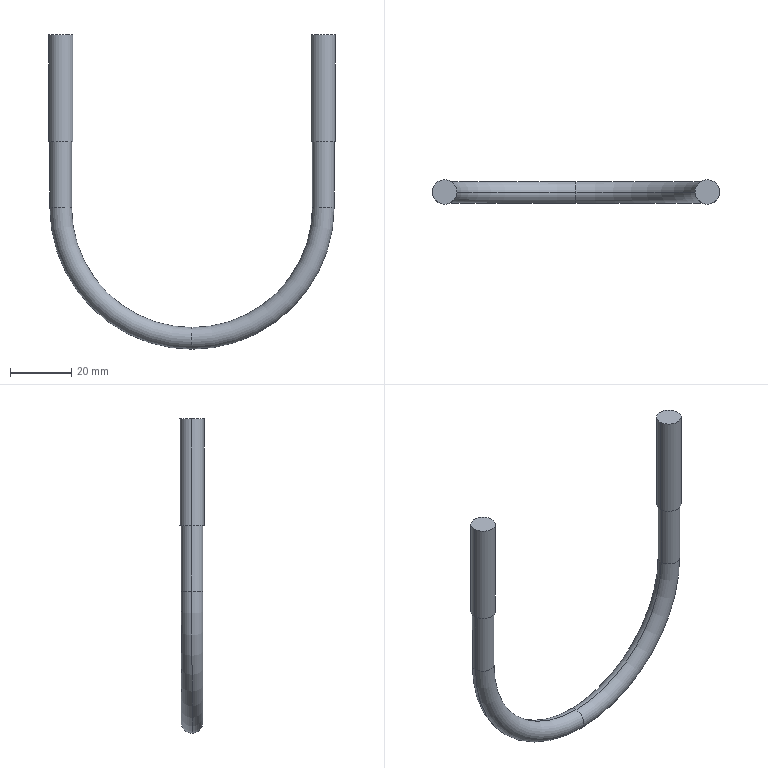Part | SolidWorks | features ICE 1, Sweep 1 | 1 solid | 16 faces | box 94 x 8 x 103 mm | volume 10565 mm3 | cylinder 8 | torus 4 | plane 4 | commonest cylinder face diameters 7.1 x4 8 x4
STEP:
#1=CARTESIAN_POINT('',(43.,0.,-103.));
#2=VERTEX_POINT('',#1);
#3=CARTESIAN_POINT('',(43.,0.,-95.9));
#4=VERTEX_POINT('',#3);
#5=CARTESIAN_POINT('',(43.,0.,-99.45));
#6=DIRECTION('',(-1.,0.,0.));
#7=DIRECTION('',(0.,0.,1.));
#8=AXIS2_PLACEMENT_3D('',#5,#6,#7);
#9=CIRCLE('',#8,3.55);
#10=EDGE_CURVE('',#2,#4,#9,.T.);
#11=ORIENTED_EDGE('',*,*,#10,.F.);
#12=CARTESIAN_POINT('',(89.55,0.,-56.45));
#13=VERTEX_POINT('',#12);
#14=CARTESIAN_POINT('',(43.,0.,-56.45));
#15=DIRECTION('',(0.,-1.,0.));
#16=DIRECTION('',(0.,0.,-1.));
#17=AXIS2_PLACEMENT_3D('',#14,#15,#16);
#18=CIRCLE('',#17,46.55);
#19=EDGE_CURVE('',#2,#13,#18,.T.);
#20=ORIENTED_EDGE('',*,*,#19,.T.);
#21=CARTESIAN_POINT('',(82.45,0.,-56.45));
#22=VERTEX_POINT('',#21);
#23=CARTESIAN_POINT('',(86.,0.,-56.45));
#24=DIRECTION('',(0.,0.,-1.));
#25=DIRECTION('',(-1.,0.,0.));
#26=AXIS2_PLACEMENT_3D('',#23,#24,#25);
#27=CIRCLE('',#26,3.55);
#28=EDGE_CURVE('',#13,#22,#27,.T.);
#29=ORIENTED_EDGE('',*,*,#28,.T.);
#30=CARTESIAN_POINT('',(43.,0.,-56.45));
#31=DIRECTION('',(0.,-1.,0.));
#32=DIRECTION('',(0.,0.,-1.));
#33=AXIS2_PLACEMENT_3D('',#30,#31,#32);
#34=CIRCLE('',#33,39.45);
#35=EDGE_CURVE('',#4,#22,#34,.T.);
#36=ORIENTED_EDGE('',*,*,#35,.F.);
#37=EDGE_LOOP('',(#11,#20,#29,#36));
#38=FACE_OUTER_BOUND('',#37,.T.);
#39=CARTESIAN_POINT('',(43.,0.,-56.45));
#40=DIRECTION('',(0.,-1.,0.));
#41=DIRECTION('',(0.,0.,-1.));
#42=AXIS2_PLACEMENT_3D('',#39,#40,#41);
#43=TOROIDAL_SURFACE('',#42,43.,3.55);
#44=ADVANCED_FACE('',(#38),#43,.T.);
#45=CARTESIAN_POINT('',(-3.55,0.,-56.45));
#46=VERTEX_POINT('',#45);
#47=CARTESIAN_POINT('',(3.55,0.,-56.45));
#48=VERTEX_POINT('',#47);
#49=CARTESIAN_POINT('',(0.,0.,-56.45));
#50=DIRECTION('',(0.,0.,1.));
#51=DIRECTION('',(1.,0.,0.));
#52=AXIS2_PLACEMENT_3D('',#49,#50,#51);
#53=CIRCLE('',#52,3.55);
#54=EDGE_CURVE('',#46,#48,#53,.T.);
#55=ORIENTED_EDGE('',*,*,#54,.F.);
#56=CARTESIAN_POINT('',(43.,0.,-56.45));
#57=DIRECTION('',(0.,-1.,0.));
#58=DIRECTION('',(0.,0.,-1.));
#59=AXIS2_PLACEMENT_3D('',#56,#57,#58);
#60=CIRCLE('',#59,46.55);
#61=EDGE_CURVE('',#46,#2,#60,.T.);
#62=ORIENTED_EDGE('',*,*,#61,.T.);
#63=ORIENTED_EDGE('',*,*,#10,.T.);
#64=CARTESIAN_POINT('',(43.,0.,-56.45));
#65=DIRECTION('',(0.,-1.,0.));
#66=DIRECTION('',(0.,0.,-1.));
#67=AXIS2_PLACEMENT_3D('',#64,#65,#66);
#68=CIRCLE('',#67,39.45);
#69=EDGE_CURVE('',#48,#4,#68,.T.);
#70=ORIENTED_EDGE('',*,*,#69,.F.);
#71=EDGE_LOOP('',(#55,#62,#63,#70));
#72=FACE_OUTER_BOUND('',#71,.T.);
#73=CARTESIAN_POINT('',(43.,0.,-56.45));
#74=DIRECTION('',(0.,-1.,0.));
#75=DIRECTION('',(0.,0.,-1.));
#76=AXIS2_PLACEMENT_3D('',#73,#74,#75);
#77=TOROIDAL_SURFACE('',#76,43.,3.55);
#78=ADVANCED_FACE('',(#72),#77,.T.);
#79=CARTESIAN_POINT('',(90.,0.,-35.));
#80=VERTEX_POINT('',#79);
#81=CARTESIAN_POINT('',(82.,0.,-35.));
#82=VERTEX_POINT('',#81);
#83=CARTESIAN_POINT('',(86.,0.,-35.));
#84=DIRECTION('',(0.,0.,1.));
#85=DIRECTION('',(1.,0.,0.));
#86=AXIS2_PLACEMENT_3D('',#83,#84,#85);
#87=CIRCLE('',#86,4.);
#88=EDGE_CURVE('',#80,#82,#87,.T.);
#89=ORIENTED_EDGE('',*,*,#88,.T.);
#90=CARTESIAN_POINT('',(82.,0.,0.));
#91=VERTEX_POINT('',#90);
#92=CARTESIAN_POINT('',(82.,0.,-35.));
#93=DIRECTION('',(0.,0.,1.));
#94=VECTOR('',#93,1000.);
#95=LINE('',#92,#94);
#96=EDGE_CURVE('',#82,#91,#95,.T.);
#97=ORIENTED_EDGE('',*,*,#96,.T.);
#98=CARTESIAN_POINT('',(90.,0.,0.));
#99=VERTEX_POINT('',#98);
#100=CARTESIAN_POINT('',(86.,0.,0.));
#101=DIRECTION('',(0.,0.,1.));
#102=DIRECTION('',(1.,0.,0.));
#103=AXIS2_PLACEMENT_3D('',#100,#101,#102);
#104=CIRCLE('',#103,4.);
#105=EDGE_CURVE('',#99,#91,#104,.T.);
#106=ORIENTED_EDGE('',*,*,#105,.F.);
#107=CARTESIAN_POINT('',(90.,0.,-35.));
#108=DIRECTION('',(0.,0.,1.));
#109=VECTOR('',#108,1000.);
#110=LINE('',#107,#109);
#111=EDGE_CURVE('',#80,#99,#110,.T.);
#112=ORIENTED_EDGE('',*,*,#111,.F.);
#113=EDGE_LOOP('',(#89,#97,#106,#112));
#114=FACE_OUTER_BOUND('',#113,.T.);
#115=CARTESIAN_POINT('',(86.,0.,-35.));
#116=DIRECTION('',(0.,0.,1.));
#117=DIRECTION('',(1.,0.,0.));
#118=AXIS2_PLACEMENT_3D('',#115,#116,#117);
#119=CYLINDRICAL_SURFACE('',#118,4.);
#120=ADVANCED_FACE('',(#114),#119,.T.);
#121=CARTESIAN_POINT('',(4.,0.,-35.));
#122=VERTEX_POINT('',#121);
#123=CARTESIAN_POINT('',(-4.,0.,-35.));
#124=VERTEX_POINT('',#123);
#125=CARTESIAN_POINT('',(0.,0.,-35.));
#126=DIRECTION('',(0.,0.,1.));
#127=DIRECTION('',(1.,0.,0.));
#128=AXIS2_PLACEMENT_3D('',#125,#126,#127);
#129=CIRCLE('',#128,4.);
#130=EDGE_CURVE('',#122,#124,#129,.T.);
#131=ORIENTED_EDGE('',*,*,#130,.T.);
#132=CARTESIAN_POINT('',(-4.,0.,0.));
#133=VERTEX_POINT('',#132);
#134=CARTESIAN_POINT('',(-4.,0.,-35.));
#135=DIRECTION('',(0.,0.,1.));
#136=VECTOR('',#135,1000.);
#137=LINE('',#134,#136);
#138=EDGE_CURVE('',#124,#133,#137,.T.);
#139=ORIENTED_EDGE('',*,*,#138,.T.);
#140=CARTESIAN_POINT('',(4.,0.,0.));
#141=VERTEX_POINT('',#140);
#142=CARTESIAN_POINT('',(0.,0.,0.));
#143=DIRECTION('',(0.,0.,1.));
#144=DIRECTION('',(1.,0.,0.));
#145=AXIS2_PLACEMENT_3D('',#142,#143,#144);
#146=CIRCLE('',#145,4.);
#147=EDGE_CURVE('',#141,#133,#146,.T.);
#148=ORIENTED_EDGE('',*,*,#147,.F.);
#149=CARTESIAN_POINT('',(4.,0.,-35.));
#150=DIRECTION('',(0.,0.,1.));
#151=VECTOR('',#150,1000.);
#152=LINE('',#149,#151);
#153=EDGE_CURVE('',#122,#141,#152,.T.);
#154=ORIENTED_EDGE('',*,*,#153,.F.);
#155=EDGE_LOOP('',(#131,#139,#148,#154));
#156=FACE_OUTER_BOUND('',#155,.T.);
#157=CARTESIAN_POINT('',(0.,0.,-35.));
#158=DIRECTION('',(0.,0.,1.));
#159=DIRECTION('',(1.,0.,0.));
#160=AXIS2_PLACEMENT_3D('',#157,#158,#159);
#161=CYLINDRICAL_SURFACE('',#160,4.);
#162=ADVANCED_FACE('',(#156),#161,.T.);
#163=ORIENTED_EDGE('',*,*,#61,.F.);
#164=CARTESIAN_POINT('',(0.,0.,-56.45));
#165=DIRECTION('',(0.,0.,1.));
#166=DIRECTION('',(1.,0.,0.));
#167=AXIS2_PLACEMENT_3D('',#164,#165,#166);
#168=CIRCLE('',#167,3.55);
#169=EDGE_CURVE('',#48,#46,#168,.T.);
#170=ORIENTED_EDGE('',*,*,#169,.F.);
#171=ORIENTED_EDGE('',*,*,#69,.T.);
#172=CARTESIAN_POINT('',(43.,0.,-99.45));
#173=DIRECTION('',(-1.,0.,0.));
#174=DIRECTION('',(0.,0.,1.));
#175=AXIS2_PLACEMENT_3D('',#172,#173,#174);
#176=CIRCLE('',#175,3.55);
#177=EDGE_CURVE('',#4,#2,#176,.T.);
#178=ORIENTED_EDGE('',*,*,#177,.T.);
#179=EDGE_LOOP('',(#163,#170,#171,#178));
#180=FACE_OUTER_BOUND('',#179,.T.);
#181=CARTESIAN_POINT('',(43.,0.,-56.45));
#182=DIRECTION('',(0.,-1.,0.));
#183=DIRECTION('',(0.,0.,-1.));
#184=AXIS2_PLACEMENT_3D('',#181,#182,#183);
#185=TOROIDAL_SURFACE('',#184,43.,3.55);
#186=ADVANCED_FACE('',(#180),#185,.T.);
#187=CARTESIAN_POINT('',(3.55,0.,-35.));
#188=VERTEX_POINT('',#187);
#189=CARTESIAN_POINT('',(-3.55,0.,-35.));
#190=VERTEX_POINT('',#189);
#191=CARTESIAN_POINT('',(0.,0.,-35.));
#192=DIRECTION('',(0.,0.,1.));
#193=DIRECTION('',(1.,0.,0.));
#194=AXIS2_PLACEMENT_3D('',#191,#192,#193);
#195=CIRCLE('',#194,3.55);
#196=EDGE_CURVE('',#188,#190,#195,.T.);
#197=ORIENTED_EDGE('',*,*,#196,.F.);
#198=CARTESIAN_POINT('',(3.55,0.,0.));
#199=DIRECTION('',(0.,0.,-1.));
#200=VECTOR('',#199,1000.);
#201=LINE('',#198,#200);
#202=EDGE_CURVE('',#188,#48,#201,.T.);
#203=ORIENTED_EDGE('',*,*,#202,.T.);
#204=ORIENTED_EDGE('',*,*,#169,.T.);
#205=CARTESIAN_POINT('',(-3.55,0.,0.));
#206=DIRECTION('',(0.,0.,-1.));
#207=VECTOR('',#206,1000.);
#208=LINE('',#205,#207);
#209=EDGE_CURVE('',#190,#46,#208,.T.);
#210=ORIENTED_EDGE('',*,*,#209,.F.);
#211=EDGE_LOOP('',(#197,#203,#204,#210));
#212=FACE_OUTER_BOUND('',#211,.T.);
#213=CARTESIAN_POINT('',(0.,0.,0.));
#214=DIRECTION('',(0.,0.,-1.));
#215=DIRECTION('',(-1.,0.,0.));
#216=AXIS2_PLACEMENT_3D('',#213,#214,#215);
#217=CYLINDRICAL_SURFACE('',#216,3.55);
#218=ADVANCED_FACE('',(#212),#217,.T.);
#219=CARTESIAN_POINT('',(86.,0.,-56.45));
#220=DIRECTION('',(0.,0.,-1.));
#221=DIRECTION('',(-1.,0.,0.));
#222=AXIS2_PLACEMENT_3D('',#219,#220,#221);
#223=CIRCLE('',#222,3.55);
#224=EDGE_CURVE('',#22,#13,#223,.T.);
#225=ORIENTED_EDGE('',*,*,#224,.F.);
#226=CARTESIAN_POINT('',(82.45,0.,-35.));
#227=VERTEX_POINT('',#226);
#228=CARTESIAN_POINT('',(82.45,0.,-56.45));
#229=DIRECTION('',(0.,0.,1.));
#230=VECTOR('',#229,1000.);
#231=LINE('',#228,#230);
#232=EDGE_CURVE('',#22,#227,#231,.T.);
#233=ORIENTED_EDGE('',*,*,#232,.T.);
#234=CARTESIAN_POINT('',(89.55,0.,-35.));
#235=VERTEX_POINT('',#234);
#236=CARTESIAN_POINT('',(86.,0.,-35.));
#237=DIRECTION('',(0.,0.,1.));
#238=DIRECTION('',(1.,0.,0.));
#239=AXIS2_PLACEMENT_3D('',#236,#237,#238);
#240=CIRCLE('',#239,3.55);
#241=EDGE_CURVE('',#235,#227,#240,.T.);
#242=ORIENTED_EDGE('',*,*,#241,.F.);
#243=CARTESIAN_POINT('',(89.55,0.,-56.45));
#244=DIRECTION('',(0.,0.,1.));
#245=VECTOR('',#244,1000.);
#246=LINE('',#243,#245);
#247=EDGE_CURVE('',#13,#235,#246,.T.);
#248=ORIENTED_EDGE('',*,*,#247,.F.);
#249=EDGE_LOOP('',(#225,#233,#242,#248));
#250=FACE_OUTER_BOUND('',#249,.T.);
#251=CARTESIAN_POINT('',(86.,0.,-56.45));
#252=DIRECTION('',(0.,0.,1.));
#253=DIRECTION('',(1.,0.,0.));
#254=AXIS2_PLACEMENT_3D('',#251,#252,#253);
#255=CYLINDRICAL_SURFACE('',#254,3.55);
#256=ADVANCED_FACE('',(#250),#255,.T.);
#257=ORIENTED_EDGE('',*,*,#232,.F.);
#258=ORIENTED_EDGE('',*,*,#28,.F.);
#259=ORIENTED_EDGE('',*,*,#247,.T.);
#260=CARTESIAN_POINT('',(86.,0.,-35.));
#261=DIRECTION('',(0.,0.,1.));
#262=DIRECTION('',(1.,0.,0.));
#263=AXIS2_PLACEMENT_3D('',#260,#261,#262);
#264=CIRCLE('',#263,3.55);
#265=EDGE_CURVE('',#227,#235,#264,.T.);
#266=ORIENTED_EDGE('',*,*,#265,.F.);
#267=EDGE_LOOP('',(#257,#258,#259,#266));
#268=FACE_OUTER_BOUND('',#267,.T.);
#269=CARTESIAN_POINT('',(86.,0.,-56.45));
#270=DIRECTION('',(0.,0.,1.));
#271=DIRECTION('',(1.,0.,0.));
#272=AXIS2_PLACEMENT_3D('',#269,#270,#271);
#273=CYLINDRICAL_SURFACE('',#272,3.55);
#274=ADVANCED_FACE('',(#268),#273,.T.);
#275=ORIENTED_EDGE('',*,*,#202,.F.);
#276=CARTESIAN_POINT('',(0.,0.,-35.));
#277=DIRECTION('',(0.,0.,1.));
#278=DIRECTION('',(1.,0.,0.));
#279=AXIS2_PLACEMENT_3D('',#276,#277,#278);
#280=CIRCLE('',#279,3.55);
#281=EDGE_CURVE('',#190,#188,#280,.T.);
#282=ORIENTED_EDGE('',*,*,#281,.F.);
#283=ORIENTED_EDGE('',*,*,#209,.T.);
#284=ORIENTED_EDGE('',*,*,#54,.T.);
#285=EDGE_LOOP('',(#275,#282,#283,#284));
#286=FACE_OUTER_BOUND('',#285,.T.);
#287=CARTESIAN_POINT('',(0.,0.,0.));
#288=DIRECTION('',(0.,0.,-1.));
#289=DIRECTION('',(-1.,0.,0.));
#290=AXIS2_PLACEMENT_3D('',#287,#288,#289);
#291=CYLINDRICAL_SURFACE('',#290,3.55);
#292=ADVANCED_FACE('',(#286),#291,.T.);
#293=ORIENTED_EDGE('',*,*,#19,.F.);
#294=ORIENTED_EDGE('',*,*,#177,.F.);
#295=ORIENTED_EDGE('',*,*,#35,.T.);
#296=ORIENTED_EDGE('',*,*,#224,.T.);
#297=EDGE_LOOP('',(#293,#294,#295,#296));
#298=FACE_OUTER_BOUND('',#297,.T.);
#299=CARTESIAN_POINT('',(43.,0.,-56.45));
#300=DIRECTION('',(0.,-1.,0.));
#301=DIRECTION('',(0.,0.,-1.));
#302=AXIS2_PLACEMENT_3D('',#299,#300,#301);
#303=TOROIDAL_SURFACE('',#302,43.,3.55);
#304=ADVANCED_FACE('',(#298),#303,.T.);
#305=ORIENTED_EDGE('',*,*,#138,.F.);
#306=CARTESIAN_POINT('',(0.,0.,-35.));
#307=DIRECTION('',(0.,0.,1.));
#308=DIRECTION('',(1.,0.,0.));
#309=AXIS2_PLACEMENT_3D('',#306,#307,#308);
#310=CIRCLE('',#309,4.);
#311=EDGE_CURVE('',#124,#122,#310,.T.);
#312=ORIENTED_EDGE('',*,*,#311,.T.);
#313=ORIENTED_EDGE('',*,*,#153,.T.);
#314=CARTESIAN_POINT('',(0.,0.,0.));
#315=DIRECTION('',(0.,0.,1.));
#316=DIRECTION('',(1.,0.,0.));
#317=AXIS2_PLACEMENT_3D('',#314,#315,#316);
#318=CIRCLE('',#317,4.);
#319=EDGE_CURVE('',#133,#141,#318,.T.);
#320=ORIENTED_EDGE('',*,*,#319,.F.);
#321=EDGE_LOOP('',(#305,#312,#313,#320));
#322=FACE_OUTER_BOUND('',#321,.T.);
#323=CARTESIAN_POINT('',(0.,0.,-35.));
#324=DIRECTION('',(0.,0.,1.));
#325=DIRECTION('',(1.,0.,0.));
#326=AXIS2_PLACEMENT_3D('',#323,#324,#325);
#327=CYLINDRICAL_SURFACE('',#326,4.);
#328=ADVANCED_FACE('',(#322),#327,.T.);
#329=ORIENTED_EDGE('',*,*,#281,.T.);
#330=ORIENTED_EDGE('',*,*,#196,.T.);
#331=EDGE_LOOP('',(#329,#330));
#332=FACE_BOUND('',#331,.T.);
#333=ORIENTED_EDGE('',*,*,#130,.F.);
#334=ORIENTED_EDGE('',*,*,#311,.F.);
#335=EDGE_LOOP('',(#333,#334));
#336=FACE_OUTER_BOUND('',#335,.T.);
#337=CARTESIAN_POINT('',(0.,0.,-35.));
#338=DIRECTION('',(0.,0.,1.));
#339=DIRECTION('',(1.,0.,0.));
#340=AXIS2_PLACEMENT_3D('',#337,#338,#339);
#341=PLANE('',#340);
#342=ADVANCED_FACE('',(#332,#336),#341,.F.);
#343=ORIENTED_EDGE('',*,*,#147,.T.);
#344=ORIENTED_EDGE('',*,*,#319,.T.);
#345=EDGE_LOOP('',(#343,#344));
#346=FACE_OUTER_BOUND('',#345,.T.);
#347=CARTESIAN_POINT('',(0.,0.,0.));
#348=DIRECTION('',(0.,0.,1.));
#349=DIRECTION('',(1.,0.,0.));
#350=AXIS2_PLACEMENT_3D('',#347,#348,#349);
#351=PLANE('',#350);
#352=ADVANCED_FACE('',(#346),#351,.T.);
#353=ORIENTED_EDGE('',*,*,#96,.F.);
#354=CARTESIAN_POINT('',(86.,0.,-35.));
#355=DIRECTION('',(0.,0.,1.));
#356=DIRECTION('',(1.,0.,0.));
#357=AXIS2_PLACEMENT_3D('',#354,#355,#356);
#358=CIRCLE('',#357,4.);
#359=EDGE_CURVE('',#82,#80,#358,.T.);
#360=ORIENTED_EDGE('',*,*,#359,.T.);
#361=ORIENTED_EDGE('',*,*,#111,.T.);
#362=CARTESIAN_POINT('',(86.,0.,0.));
#363=DIRECTION('',(0.,0.,1.));
#364=DIRECTION('',(1.,0.,0.));
#365=AXIS2_PLACEMENT_3D('',#362,#363,#364);
#366=CIRCLE('',#365,4.);
#367=EDGE_CURVE('',#91,#99,#366,.T.);
#368=ORIENTED_EDGE('',*,*,#367,.F.);
#369=EDGE_LOOP('',(#353,#360,#361,#368));
#370=FACE_OUTER_BOUND('',#369,.T.);
#371=CARTESIAN_POINT('',(86.,0.,-35.));
#372=DIRECTION('',(0.,0.,1.));
#373=DIRECTION('',(1.,0.,0.));
#374=AXIS2_PLACEMENT_3D('',#371,#372,#373);
#375=CYLINDRICAL_SURFACE('',#374,4.);
#376=ADVANCED_FACE('',(#370),#375,.T.);
#377=ORIENTED_EDGE('',*,*,#241,.T.);
#378=ORIENTED_EDGE('',*,*,#265,.T.);
#379=EDGE_LOOP('',(#377,#378));
#380=FACE_BOUND('',#379,.T.);
#381=ORIENTED_EDGE('',*,*,#88,.F.);
#382=ORIENTED_EDGE('',*,*,#359,.F.);
#383=EDGE_LOOP('',(#381,#382));
#384=FACE_OUTER_BOUND('',#383,.T.);
#385=CARTESIAN_POINT('',(86.,0.,-35.));
#386=DIRECTION('',(0.,0.,1.));
#387=DIRECTION('',(1.,0.,0.));
#388=AXIS2_PLACEMENT_3D('',#385,#386,#387);
#389=PLANE('',#388);
#390=ADVANCED_FACE('',(#380,#384),#389,.F.);
#391=ORIENTED_EDGE('',*,*,#105,.T.);
#392=ORIENTED_EDGE('',*,*,#367,.T.);
#393=EDGE_LOOP('',(#391,#392));
#394=FACE_OUTER_BOUND('',#393,.T.);
#395=CARTESIAN_POINT('',(86.,0.,0.));
#396=DIRECTION('',(0.,0.,-1.));
#397=DIRECTION('',(-1.,0.,0.));
#398=AXIS2_PLACEMENT_3D('',#395,#396,#397);
#399=PLANE('',#398);
#400=ADVANCED_FACE('',(#394),#399,.F.);
#401=CLOSED_SHELL('',(#44,#78,#120,#162,#186,#218,#256,#274,#292,#304,#328,#342,#352,#376,#390,#400));
#402=MANIFOLD_SOLID_BREP('',#401);
#403=CARTESIAN_POINT('',(0.,0.,0.));
#404=DIRECTION('',(0.,0.,1.));
#405=DIRECTION('',(1.,0.,0.));
#406=AXIS2_PLACEMENT_3D('',#403,#404,#405);
#407=(LENGTH_UNIT()NAMED_UNIT(*)SI_UNIT(.MILLI.,.METRE.));
#408=UNCERTAINTY_MEASURE_WITH_UNIT(LENGTH_MEASURE(0.00001),#407,'','');
#409=(NAMED_UNIT(*)PLANE_ANGLE_UNIT()SI_UNIT($,.RADIAN.));
#410=(NAMED_UNIT(*)SI_UNIT($,.STERADIAN.)SOLID_ANGLE_UNIT());
#411=(GEOMETRIC_REPRESENTATION_CONTEXT(3)GLOBAL_UNCERTAINTY_ASSIGNED_CONTEXT((#408))GLOBAL_UNIT_ASSIGNED_CONTEXT((#407,#409,#410))REPRESENTATION_CONTEXT('',''));
#412=ADVANCED_BREP_SHAPE_REPRESENTATION('',(#402,#406),#411);